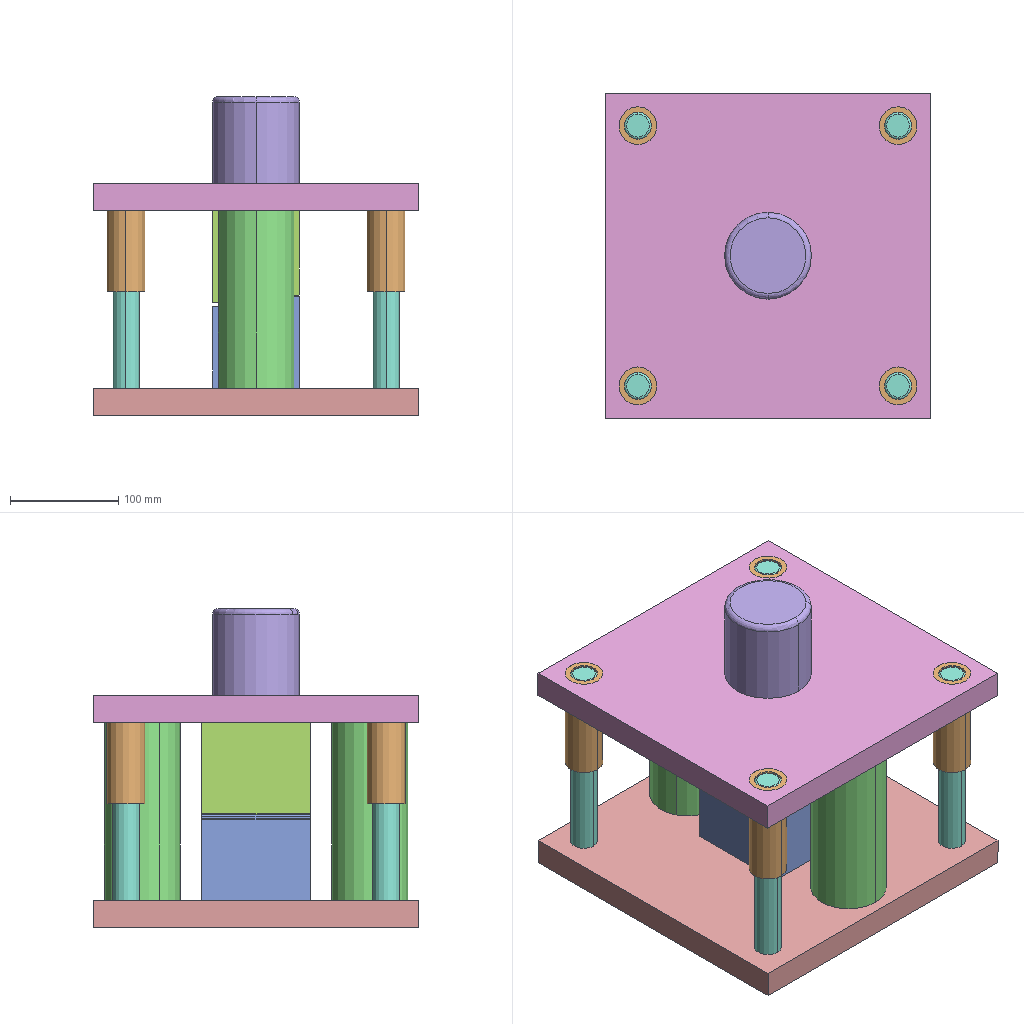Assembly | SolidWorks | 8 different items | 15 placed | box 300 x 300 x 294 mm
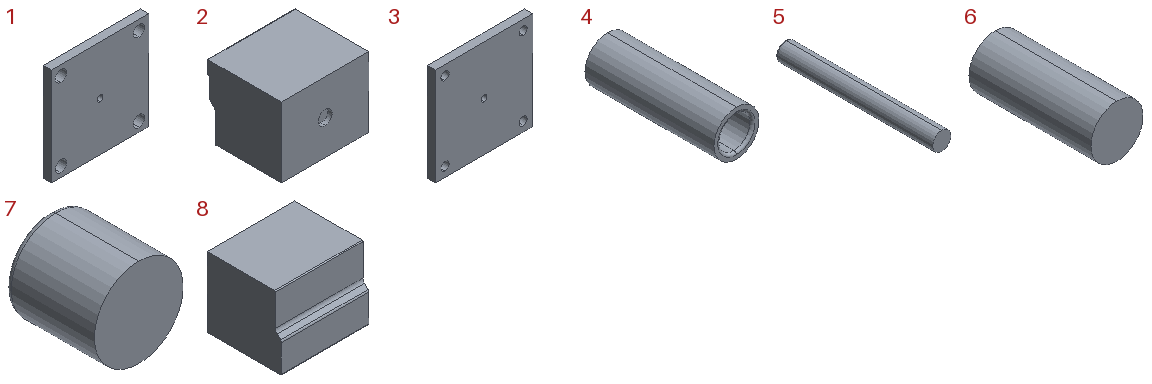Parts list (item | quantity | size | volume | features):
1 | x1 | 300 x 25 x 300 mm | 2147427 mm3 | features FlatPattern 1, SMBaseFlange 1, SheetMetal 1
2 | x1 | 100 x 85 x 80 mm | 636588 mm3 | features FlatPattern 1, ICE 1, SMBaseFlange 1, SheetMetal 1
3 | x1 | 300 x 25 x 300 mm | 2194551 mm3 | features FlatPattern 1, SMBaseFlange 1, SheetMetal 1
4 | x4 | 35 x 100 x 35 mm | 47054 mm3 | features Extrusion 1, Fillet 1
5 | x4 | 25 x 213.5 x 25 mm | 104737 mm3 | features Extrusion 1, Fillet 1
6 | x2 | 70 x 163.9 x 70 mm | 630761 mm3 | features Extrusion 1
7 | x1 | 80 x 80 x 80 mm | 400813 mm3 | features Extrusion 1, Fillet 1
8 | x1 | 100 x 85 x 80 mm | 649829 mm3 | features FlatPattern 1, ICE 1, SMBaseFlange 1, SheetMetal 1
Mates (type | each side: item.copy, entity, surface, feature):
Coincident | 3.1 face plane Base-Flange1 | 2.1 face plane Base-Flange1
Concentric | 3.1 face cylinder Base-Flange1 | 2.1 face cylinder Cut-Extrude1
Parallel | 3.1 face plane Base-Flange1 | 2.1 face plane Base-Flange1
DistanceDim | 2.1 face plane Base-Flange1 | 8.1 face plane Base-Flange1
Coincident | 2.1 face plane Base-Flange1 | 8.1 face plane Base-Flange1 | 2 times
Coincident | 8.1 face plane Base-Flange1 | 1.1 face plane Base-Flange1
Concentric | 8.1 face cylinder Cut-Extrude1 | 1.1 face cylinder Base-Flange1
Concentric | 3.1 face cylinder Base-Flange1 | 1.1 face cylinder Base-Flange1
Concentric | 3.1 face cylinder Base-Flange1 | 5.1 face cylinder Boss-Extrude1
Coincident | 3.1 face plane Base-Flange1 | 5.1 face plane Boss-Extrude1
Concentric | 3.1 face cylinder Base-Flange1 | 5.2 face cylinder Boss-Extrude1
Coincident | 3.1 face plane Base-Flange1 | 5.2 face plane Boss-Extrude1
Concentric | 3.1 face cylinder Base-Flange1 | 5.3 face cylinder Boss-Extrude1
Coincident | 3.1 face plane Base-Flange1 | 5.3 face plane Boss-Extrude1
Concentric | 1.1 face cylinder Base-Flange1 | 4.1 face cylinder Boss-Extrude1
Coincident | 1.1 face plane Base-Flange1 | 4.1 face plane Boss-Extrude1
Concentric | 1.1 face cylinder Base-Flange1 | 4.2 face cylinder Boss-Extrude1
Coincident | 1.1 face plane Base-Flange1 | 4.2 face plane Boss-Extrude1
Concentric | 1.1 face cylinder Base-Flange1 | 4.3 face cylinder Boss-Extrude1
Coincident | 1.1 face plane Base-Flange1 | 4.3 face plane Boss-Extrude1
Coincident | 1.1 face plane Base-Flange1 | 7.1 face plane Boss-Extrude1
Concentric | 1.1 face cylinder Base-Flange1 | 7.1 face cylinder Boss-Extrude1
Concentric | 3.1 face cylinder Base-Flange1 | 5.4 face cylinder Boss-Extrude1
Coincident | 3.1 face plane Base-Flange1 | 5.4 face plane Boss-Extrude1
Concentric | 1.1 face cylinder Base-Flange1 | 4.4 face cylinder Boss-Extrude1
Coincident | 1.1 face plane Base-Flange1 | 4.4 face plane Boss-Extrude1
Coincident | 3.1 face plane Base-Flange1 | 6.1 face plane Boss-Extrude1
DistanceDim | 6.1 face cylinder Boss-Extrude1 | 3.1 face plane Base-Flange1
DistanceDim | 3.1 face plane Base-Flange1 | 6.1 face cylinder Boss-Extrude1
Coincident | 3.1 face plane Base-Flange1 | 6.2 face plane Boss-Extrude1
DistanceDim | 3.1 face plane Base-Flange1 | 6.2 face cylinder Boss-Extrude1
DistanceDim | 6.2 face cylinder Boss-Extrude1 | 3.1 face plane Base-Flange1